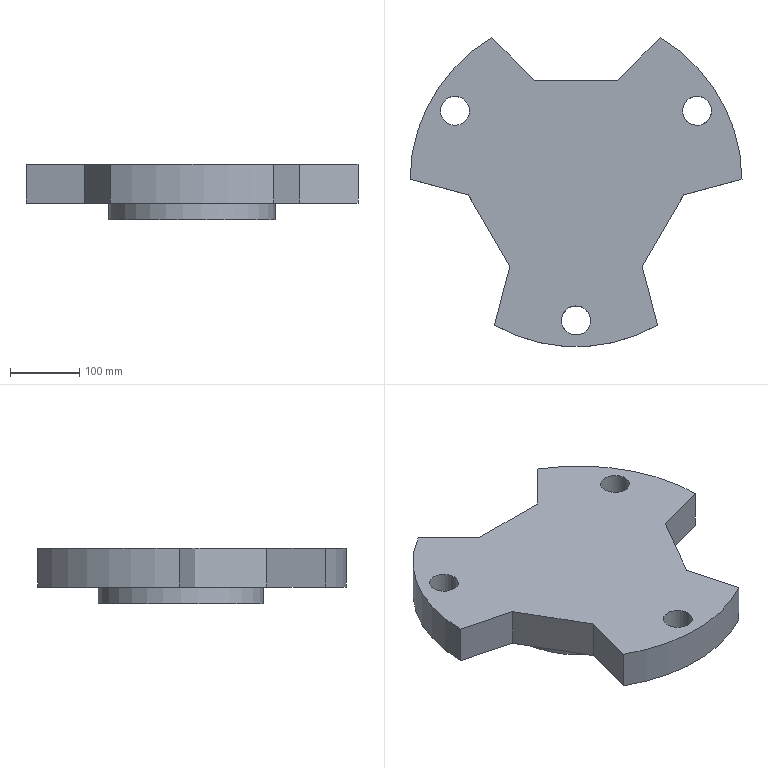Part | NX | features CYLINDER 3, DATUM_CSYS 2, EXTRUDE 1, SKETCH 1 | 1 solid | 21 faces | box 479.982 x 446.798 x 80 mm | volume 8098473 mm3 | plane 13 | cylinder 8 | commonest cylinder face diameters 42 x3 480 x3 48 x1 240 x1
STEP:
#1=CARTESIAN_POINT('',(-239.991,2.081,56.));
#2=VERTEX_POINT('',#1);
#3=CARTESIAN_POINT('',(-239.991,2.081,0.));
#4=VERTEX_POINT('',#3);
#5=CARTESIAN_POINT('',(-239.991,2.081,0.));
#6=DIRECTION('',(0.,0.,1.));
#7=VECTOR('',#6,1000.);
#8=LINE('',#5,#7);
#9=EDGE_CURVE('',#2,#4,#8,.F.);
#10=ORIENTED_EDGE('',*,*,#9,.F.);
#11=CARTESIAN_POINT('',(-121.798,206.798,56.));
#12=VERTEX_POINT('',#11);
#13=CARTESIAN_POINT('',(0.,0.,56.));
#14=DIRECTION('',(0.,0.,-1.));
#15=DIRECTION('',(1.,0.,0.));
#16=AXIS2_PLACEMENT_3D('',#13,#14,#15);
#17=CIRCLE('',#16,240.);
#18=EDGE_CURVE('',#2,#12,#17,.T.);
#19=ORIENTED_EDGE('',*,*,#18,.T.);
#20=CARTESIAN_POINT('',(-121.798,206.798,0.));
#21=VERTEX_POINT('',#20);
#22=CARTESIAN_POINT('',(-121.798,206.798,0.));
#23=DIRECTION('',(0.,0.,1.));
#24=VECTOR('',#23,1000.);
#25=LINE('',#22,#24);
#26=EDGE_CURVE('',#21,#12,#25,.T.);
#27=ORIENTED_EDGE('',*,*,#26,.F.);
#28=CARTESIAN_POINT('',(0.,0.,0.));
#29=DIRECTION('',(0.,0.,1.));
#30=DIRECTION('',(1.,0.,0.));
#31=AXIS2_PLACEMENT_3D('',#28,#29,#30);
#32=CIRCLE('',#31,240.);
#33=EDGE_CURVE('',#21,#4,#32,.T.);
#34=ORIENTED_EDGE('',*,*,#33,.T.);
#35=EDGE_LOOP('',(#10,#19,#27,#34));
#36=FACE_BOUND('',#35,.T.);
#37=CARTESIAN_POINT('',(0.,0.,0.));
#38=DIRECTION('',(0.,0.,1.));
#39=DIRECTION('',(1.,0.,0.));
#40=AXIS2_PLACEMENT_3D('',#37,#38,#39);
#41=CYLINDRICAL_SURFACE('',#40,240.);
#42=ADVANCED_FACE('',(#36),#41,.T.);
#43=CARTESIAN_POINT('',(-118.193,-208.879,0.));
#44=VERTEX_POINT('',#43);
#45=CARTESIAN_POINT('',(-118.193,-208.879,56.));
#46=VERTEX_POINT('',#45);
#47=CARTESIAN_POINT('',(-118.193,-208.879,0.));
#48=DIRECTION('',(0.,0.,1.));
#49=VECTOR('',#48,1000.);
#50=LINE('',#47,#49);
#51=EDGE_CURVE('',#44,#46,#50,.T.);
#52=ORIENTED_EDGE('',*,*,#51,.F.);
#53=CARTESIAN_POINT('',(118.193,-208.879,0.));
#54=VERTEX_POINT('',#53);
#55=CARTESIAN_POINT('',(0.,0.,0.));
#56=DIRECTION('',(0.,0.,1.));
#57=DIRECTION('',(1.,0.,0.));
#58=AXIS2_PLACEMENT_3D('',#55,#56,#57);
#59=CIRCLE('',#58,240.);
#60=EDGE_CURVE('',#44,#54,#59,.T.);
#61=ORIENTED_EDGE('',*,*,#60,.T.);
#62=CARTESIAN_POINT('',(118.193,-208.879,56.));
#63=VERTEX_POINT('',#62);
#64=CARTESIAN_POINT('',(118.193,-208.879,0.));
#65=DIRECTION('',(0.,0.,1.));
#66=VECTOR('',#65,1000.);
#67=LINE('',#64,#66);
#68=EDGE_CURVE('',#63,#54,#67,.F.);
#69=ORIENTED_EDGE('',*,*,#68,.F.);
#70=CARTESIAN_POINT('',(0.,0.,56.));
#71=DIRECTION('',(0.,0.,-1.));
#72=DIRECTION('',(1.,0.,0.));
#73=AXIS2_PLACEMENT_3D('',#70,#71,#72);
#74=CIRCLE('',#73,240.);
#75=EDGE_CURVE('',#63,#46,#74,.T.);
#76=ORIENTED_EDGE('',*,*,#75,.T.);
#77=EDGE_LOOP('',(#52,#61,#69,#76));
#78=FACE_BOUND('',#77,.T.);
#79=CARTESIAN_POINT('',(0.,0.,0.));
#80=DIRECTION('',(0.,0.,1.));
#81=DIRECTION('',(1.,0.,0.));
#82=AXIS2_PLACEMENT_3D('',#79,#80,#81);
#83=CYLINDRICAL_SURFACE('',#82,240.);
#84=ADVANCED_FACE('',(#78),#83,.T.);
#85=CARTESIAN_POINT('',(-154.,101.036,56.));
#86=VERTEX_POINT('',#85);
#87=CARTESIAN_POINT('',(-175.,101.036,56.));
#88=DIRECTION('',(0.,0.,1.));
#89=DIRECTION('',(1.,0.,0.));
#90=AXIS2_PLACEMENT_3D('',#87,#88,#89);
#91=CIRCLE('',#90,21.);
#92=EDGE_CURVE('',#86,#86,#91,.T.);
#93=ORIENTED_EDGE('',*,*,#92,.F.);
#94=EDGE_LOOP('',(#93));
#95=FACE_BOUND('',#94,.T.);
#96=CARTESIAN_POINT('',(-10.5,-183.886,56.));
#97=VERTEX_POINT('',#96);
#98=CARTESIAN_POINT('',(0.,-202.073,56.));
#99=DIRECTION('',(0.,0.,1.));
#100=DIRECTION('',(-0.5,0.866,0.));
#101=AXIS2_PLACEMENT_3D('',#98,#99,#100);
#102=CIRCLE('',#101,21.);
#103=EDGE_CURVE('',#97,#97,#102,.T.);
#104=ORIENTED_EDGE('',*,*,#103,.F.);
#105=EDGE_LOOP('',(#104));
#106=FACE_BOUND('',#105,.T.);
#107=CARTESIAN_POINT('',(164.5,82.85,56.));
#108=VERTEX_POINT('',#107);
#109=CARTESIAN_POINT('',(175.,101.036,56.));
#110=DIRECTION('',(0.,0.,1.));
#111=DIRECTION('',(-0.5,-0.866,0.));
#112=AXIS2_PLACEMENT_3D('',#109,#110,#111);
#113=CIRCLE('',#112,21.);
#114=EDGE_CURVE('',#108,#108,#113,.T.);
#115=ORIENTED_EDGE('',*,*,#114,.F.);
#116=EDGE_LOOP('',(#115));
#117=FACE_BOUND('',#116,.T.);
#118=CARTESIAN_POINT('',(-155.574,-20.538,56.));
#119=VERTEX_POINT('',#118);
#120=CARTESIAN_POINT('',(-155.574,-20.538,56.));
#121=DIRECTION('',(-0.9659,0.2588,0.));
#122=VECTOR('',#121,1000.);
#123=LINE('',#120,#122);
#124=EDGE_CURVE('',#119,#2,#123,.T.);
#125=ORIENTED_EDGE('',*,*,#124,.F.);
#126=CARTESIAN_POINT('',(-95.574,-124.462,56.));
#127=VERTEX_POINT('',#126);
#128=CARTESIAN_POINT('',(-95.574,-124.462,56.));
#129=DIRECTION('',(-0.5,0.866,0.));
#130=VECTOR('',#129,1000.);
#131=LINE('',#128,#130);
#132=EDGE_CURVE('',#127,#119,#131,.T.);
#133=ORIENTED_EDGE('',*,*,#132,.F.);
#134=CARTESIAN_POINT('',(-131.124,-257.136,56.));
#135=DIRECTION('',(0.2588,0.9659,0.));
#136=VECTOR('',#135,1000.);
#137=LINE('',#134,#136);
#138=EDGE_CURVE('',#46,#127,#137,.T.);
#139=ORIENTED_EDGE('',*,*,#138,.F.);
#140=ORIENTED_EDGE('',*,*,#75,.F.);
#141=CARTESIAN_POINT('',(95.574,-124.462,56.));
#142=VERTEX_POINT('',#141);
#143=CARTESIAN_POINT('',(95.574,-124.462,56.));
#144=DIRECTION('',(0.2588,-0.9659,0.));
#145=VECTOR('',#144,1000.);
#146=LINE('',#143,#145);
#147=EDGE_CURVE('',#142,#63,#146,.T.);
#148=ORIENTED_EDGE('',*,*,#147,.F.);
#149=CARTESIAN_POINT('',(155.574,-20.538,56.));
#150=VERTEX_POINT('',#149);
#151=CARTESIAN_POINT('',(155.574,-20.538,56.));
#152=DIRECTION('',(-0.5,-0.866,0.));
#153=VECTOR('',#152,1000.);
#154=LINE('',#151,#153);
#155=EDGE_CURVE('',#150,#142,#154,.T.);
#156=ORIENTED_EDGE('',*,*,#155,.F.);
#157=CARTESIAN_POINT('',(239.991,2.081,56.));
#158=VERTEX_POINT('',#157);
#159=CARTESIAN_POINT('',(288.248,15.011,56.));
#160=DIRECTION('',(-0.9659,-0.2588,0.));
#161=VECTOR('',#160,1000.);
#162=LINE('',#159,#161);
#163=EDGE_CURVE('',#158,#150,#162,.T.);
#164=ORIENTED_EDGE('',*,*,#163,.F.);
#165=CARTESIAN_POINT('',(121.798,206.798,56.));
#166=VERTEX_POINT('',#165);
#167=CARTESIAN_POINT('',(0.,0.,56.));
#168=DIRECTION('',(0.,0.,-1.));
#169=DIRECTION('',(1.,0.,0.));
#170=AXIS2_PLACEMENT_3D('',#167,#168,#169);
#171=CIRCLE('',#170,240.);
#172=EDGE_CURVE('',#166,#158,#171,.T.);
#173=ORIENTED_EDGE('',*,*,#172,.F.);
#174=CARTESIAN_POINT('',(60.,145.,56.));
#175=VERTEX_POINT('',#174);
#176=CARTESIAN_POINT('',(60.,145.,56.));
#177=DIRECTION('',(0.7071,0.7071,0.));
#178=VECTOR('',#177,1000.);
#179=LINE('',#176,#178);
#180=EDGE_CURVE('',#175,#166,#179,.T.);
#181=ORIENTED_EDGE('',*,*,#180,.F.);
#182=CARTESIAN_POINT('',(-60.,145.,56.));
#183=VERTEX_POINT('',#182);
#184=CARTESIAN_POINT('',(-60.,145.,56.));
#185=DIRECTION('',(1.,0.,0.));
#186=VECTOR('',#185,1000.);
#187=LINE('',#184,#186);
#188=EDGE_CURVE('',#183,#175,#187,.T.);
#189=ORIENTED_EDGE('',*,*,#188,.F.);
#190=CARTESIAN_POINT('',(-157.124,242.124,56.));
#191=DIRECTION('',(0.7071,-0.7071,0.));
#192=VECTOR('',#191,1000.);
#193=LINE('',#190,#192);
#194=EDGE_CURVE('',#12,#183,#193,.T.);
#195=ORIENTED_EDGE('',*,*,#194,.F.);
#196=ORIENTED_EDGE('',*,*,#18,.F.);
#197=EDGE_LOOP('',(#125,#133,#139,#140,#148,#156,#164,#173,#181,#189,#195,#196));
#198=FACE_BOUND('',#197,.T.);
#199=CARTESIAN_POINT('',(0.,0.,56.));
#200=DIRECTION('',(0.,0.,1.));
#201=DIRECTION('',(1.,0.,0.));
#202=AXIS2_PLACEMENT_3D('',#199,#200,#201);
#203=PLANE('',#202);
#204=ADVANCED_FACE('',(#95,#106,#117,#198),#203,.T.);
#205=CARTESIAN_POINT('',(-120.,0.,0.));
#206=VERTEX_POINT('',#205);
#207=CARTESIAN_POINT('',(0.,0.,0.));
#208=DIRECTION('',(0.,0.,-1.));
#209=DIRECTION('',(-1.,0.,0.));
#210=AXIS2_PLACEMENT_3D('',#207,#208,#209);
#211=CIRCLE('',#210,120.);
#212=EDGE_CURVE('',#206,#206,#211,.T.);
#213=ORIENTED_EDGE('',*,*,#212,.F.);
#214=EDGE_LOOP('',(#213));
#215=FACE_BOUND('',#214,.T.);
#216=CARTESIAN_POINT('',(-196.,101.036,0.));
#217=VERTEX_POINT('',#216);
#218=CARTESIAN_POINT('',(-175.,101.036,0.));
#219=DIRECTION('',(0.,0.,-1.));
#220=DIRECTION('',(-1.,0.,0.));
#221=AXIS2_PLACEMENT_3D('',#218,#219,#220);
#222=CIRCLE('',#221,21.);
#223=EDGE_CURVE('',#217,#217,#222,.T.);
#224=ORIENTED_EDGE('',*,*,#223,.F.);
#225=EDGE_LOOP('',(#224));
#226=FACE_BOUND('',#225,.T.);
#227=CARTESIAN_POINT('',(-21.,-202.073,0.));
#228=VERTEX_POINT('',#227);
#229=CARTESIAN_POINT('',(0.,-202.073,0.));
#230=DIRECTION('',(0.,0.,-1.));
#231=DIRECTION('',(-1.,0.,0.));
#232=AXIS2_PLACEMENT_3D('',#229,#230,#231);
#233=CIRCLE('',#232,21.);
#234=EDGE_CURVE('',#228,#228,#233,.T.);
#235=ORIENTED_EDGE('',*,*,#234,.F.);
#236=EDGE_LOOP('',(#235));
#237=FACE_BOUND('',#236,.T.);
#238=CARTESIAN_POINT('',(154.,101.036,0.));
#239=VERTEX_POINT('',#238);
#240=CARTESIAN_POINT('',(175.,101.036,0.));
#241=DIRECTION('',(0.,0.,-1.));
#242=DIRECTION('',(-1.,0.,0.));
#243=AXIS2_PLACEMENT_3D('',#240,#241,#242);
#244=CIRCLE('',#243,21.);
#245=EDGE_CURVE('',#239,#239,#244,.T.);
#246=ORIENTED_EDGE('',*,*,#245,.F.);
#247=EDGE_LOOP('',(#246));
#248=FACE_BOUND('',#247,.T.);
#249=CARTESIAN_POINT('',(-155.574,-20.538,0.));
#250=VERTEX_POINT('',#249);
#251=CARTESIAN_POINT('',(-15.556,-58.056,0.));
#252=DIRECTION('',(0.9659,-0.2588,0.));
#253=VECTOR('',#252,1000.);
#254=LINE('',#251,#253);
#255=EDGE_CURVE('',#4,#250,#254,.T.);
#256=ORIENTED_EDGE('',*,*,#255,.F.);
#257=ORIENTED_EDGE('',*,*,#33,.F.);
#258=CARTESIAN_POINT('',(-60.,145.,0.));
#259=VERTEX_POINT('',#258);
#260=CARTESIAN_POINT('',(42.5,42.5,0.));
#261=DIRECTION('',(-0.7071,0.7071,0.));
#262=VECTOR('',#261,1000.);
#263=LINE('',#260,#262);
#264=EDGE_CURVE('',#259,#21,#263,.T.);
#265=ORIENTED_EDGE('',*,*,#264,.F.);
#266=CARTESIAN_POINT('',(60.,145.,0.));
#267=VERTEX_POINT('',#266);
#268=CARTESIAN_POINT('',(0.,145.,0.));
#269=DIRECTION('',(-1.,0.,0.));
#270=VECTOR('',#269,1000.);
#271=LINE('',#268,#270);
#272=EDGE_CURVE('',#267,#259,#271,.T.);
#273=ORIENTED_EDGE('',*,*,#272,.F.);
#274=CARTESIAN_POINT('',(121.798,206.798,0.));
#275=VERTEX_POINT('',#274);
#276=CARTESIAN_POINT('',(-42.5,42.5,0.));
#277=DIRECTION('',(-0.7071,-0.7071,0.));
#278=VECTOR('',#277,1000.);
#279=LINE('',#276,#278);
#280=EDGE_CURVE('',#275,#267,#279,.T.);
#281=ORIENTED_EDGE('',*,*,#280,.F.);
#282=CARTESIAN_POINT('',(239.991,2.081,0.));
#283=VERTEX_POINT('',#282);
#284=CARTESIAN_POINT('',(0.,0.,0.));
#285=DIRECTION('',(0.,0.,1.));
#286=DIRECTION('',(1.,0.,0.));
#287=AXIS2_PLACEMENT_3D('',#284,#285,#286);
#288=CIRCLE('',#287,240.);
#289=EDGE_CURVE('',#283,#275,#288,.T.);
#290=ORIENTED_EDGE('',*,*,#289,.F.);
#291=CARTESIAN_POINT('',(155.574,-20.538,0.));
#292=VERTEX_POINT('',#291);
#293=CARTESIAN_POINT('',(15.556,-58.056,0.));
#294=DIRECTION('',(0.9659,0.2588,0.));
#295=VECTOR('',#294,1000.);
#296=LINE('',#293,#295);
#297=EDGE_CURVE('',#292,#283,#296,.T.);
#298=ORIENTED_EDGE('',*,*,#297,.F.);
#299=CARTESIAN_POINT('',(95.574,-124.462,0.));
#300=VERTEX_POINT('',#299);
#301=CARTESIAN_POINT('',(125.574,-72.5,0.));
#302=DIRECTION('',(0.5,0.866,0.));
#303=VECTOR('',#302,1000.);
#304=LINE('',#301,#303);
#305=EDGE_CURVE('',#300,#292,#304,.T.);
#306=ORIENTED_EDGE('',*,*,#305,.F.);
#307=CARTESIAN_POINT('',(58.056,15.556,0.));
#308=DIRECTION('',(-0.2588,0.9659,0.));
#309=VECTOR('',#308,1000.);
#310=LINE('',#307,#309);
#311=EDGE_CURVE('',#54,#300,#310,.T.);
#312=ORIENTED_EDGE('',*,*,#311,.F.);
#313=ORIENTED_EDGE('',*,*,#60,.F.);
#314=CARTESIAN_POINT('',(-95.574,-124.462,0.));
#315=VERTEX_POINT('',#314);
#316=CARTESIAN_POINT('',(-58.056,15.556,0.));
#317=DIRECTION('',(-0.2588,-0.9659,0.));
#318=VECTOR('',#317,1000.);
#319=LINE('',#316,#318);
#320=EDGE_CURVE('',#315,#44,#319,.T.);
#321=ORIENTED_EDGE('',*,*,#320,.F.);
#322=CARTESIAN_POINT('',(-125.574,-72.5,0.));
#323=DIRECTION('',(0.5,-0.866,0.));
#324=VECTOR('',#323,1000.);
#325=LINE('',#322,#324);
#326=EDGE_CURVE('',#250,#315,#325,.T.);
#327=ORIENTED_EDGE('',*,*,#326,.F.);
#328=EDGE_LOOP('',(#256,#257,#265,#273,#281,#290,#298,#306,#312,#313,#321,#327));
#329=FACE_BOUND('',#328,.T.);
#330=CARTESIAN_POINT('',(0.,0.,0.));
#331=DIRECTION('',(0.,0.,-1.));
#332=DIRECTION('',(-1.,0.,0.));
#333=AXIS2_PLACEMENT_3D('',#330,#331,#332);
#334=PLANE('',#333);
#335=ADVANCED_FACE('',(#215,#226,#237,#248,#329),#334,.T.);
#336=CARTESIAN_POINT('',(121.798,206.798,0.));
#337=DIRECTION('',(0.,0.,1.));
#338=VECTOR('',#337,1000.);
#339=LINE('',#336,#338);
#340=EDGE_CURVE('',#166,#275,#339,.F.);
#341=ORIENTED_EDGE('',*,*,#340,.F.);
#342=ORIENTED_EDGE('',*,*,#172,.T.);
#343=CARTESIAN_POINT('',(239.991,2.081,0.));
#344=DIRECTION('',(0.,0.,1.));
#345=VECTOR('',#344,1000.);
#346=LINE('',#343,#345);
#347=EDGE_CURVE('',#283,#158,#346,.T.);
#348=ORIENTED_EDGE('',*,*,#347,.F.);
#349=ORIENTED_EDGE('',*,*,#289,.T.);
#350=EDGE_LOOP('',(#341,#342,#348,#349));
#351=FACE_BOUND('',#350,.T.);
#352=CARTESIAN_POINT('',(0.,0.,0.));
#353=DIRECTION('',(0.,0.,1.));
#354=DIRECTION('',(1.,0.,0.));
#355=AXIS2_PLACEMENT_3D('',#352,#353,#354);
#356=CYLINDRICAL_SURFACE('',#355,240.);
#357=ADVANCED_FACE('',(#351),#356,.T.);
#358=ORIENTED_EDGE('',*,*,#311,.T.);
#359=CARTESIAN_POINT('',(95.574,-124.462,-19.));
#360=DIRECTION('',(0.,0.,1.));
#361=VECTOR('',#360,1000.);
#362=LINE('',#359,#361);
#363=EDGE_CURVE('',#142,#300,#362,.F.);
#364=ORIENTED_EDGE('',*,*,#363,.F.);
#365=ORIENTED_EDGE('',*,*,#147,.T.);
#366=ORIENTED_EDGE('',*,*,#68,.T.);
#367=EDGE_LOOP('',(#358,#364,#365,#366));
#368=FACE_BOUND('',#367,.T.);
#369=CARTESIAN_POINT('',(95.574,-124.462,-19.));
#370=DIRECTION('',(-0.9659,-0.2588,0.));
#371=DIRECTION('',(0.2588,-0.9659,0.));
#372=AXIS2_PLACEMENT_3D('',#369,#370,#371);
#373=PLANE('',#372);
#374=ADVANCED_FACE('',(#368),#373,.F.);
#375=ORIENTED_EDGE('',*,*,#297,.T.);
#376=ORIENTED_EDGE('',*,*,#347,.T.);
#377=ORIENTED_EDGE('',*,*,#163,.T.);
#378=CARTESIAN_POINT('',(155.574,-20.538,-19.));
#379=DIRECTION('',(0.,0.,1.));
#380=VECTOR('',#379,1000.);
#381=LINE('',#378,#380);
#382=EDGE_CURVE('',#150,#292,#381,.F.);
#383=ORIENTED_EDGE('',*,*,#382,.T.);
#384=EDGE_LOOP('',(#375,#376,#377,#383));
#385=FACE_BOUND('',#384,.T.);
#386=CARTESIAN_POINT('',(288.248,15.011,-19.));
#387=DIRECTION('',(-0.2588,0.9659,0.));
#388=DIRECTION('',(-0.9659,-0.2588,0.));
#389=AXIS2_PLACEMENT_3D('',#386,#387,#388);
#390=PLANE('',#389);
#391=ADVANCED_FACE('',(#385),#390,.F.);
#392=ORIENTED_EDGE('',*,*,#305,.T.);
#393=ORIENTED_EDGE('',*,*,#382,.F.);
#394=ORIENTED_EDGE('',*,*,#155,.T.);
#395=ORIENTED_EDGE('',*,*,#363,.T.);
#396=EDGE_LOOP('',(#392,#393,#394,#395));
#397=FACE_BOUND('',#396,.T.);
#398=CARTESIAN_POINT('',(155.574,-20.538,-19.));
#399=DIRECTION('',(-0.866,0.5,0.));
#400=DIRECTION('',(-0.5,-0.866,0.));
#401=AXIS2_PLACEMENT_3D('',#398,#399,#400);
#402=PLANE('',#401);
#403=ADVANCED_FACE('',(#397),#402,.F.);
#404=ORIENTED_EDGE('',*,*,#264,.T.);
#405=ORIENTED_EDGE('',*,*,#26,.T.);
#406=ORIENTED_EDGE('',*,*,#194,.T.);
#407=CARTESIAN_POINT('',(-60.,145.,-19.));
#408=DIRECTION('',(0.,0.,1.));
#409=VECTOR('',#408,1000.);
#410=LINE('',#407,#409);
#411=EDGE_CURVE('',#183,#259,#410,.F.);
#412=ORIENTED_EDGE('',*,*,#411,.T.);
#413=EDGE_LOOP('',(#404,#405,#406,#412));
#414=FACE_BOUND('',#413,.T.);
#415=CARTESIAN_POINT('',(-157.124,242.124,-19.));
#416=DIRECTION('',(-0.7071,-0.7071,0.));
#417=DIRECTION('',(0.7071,-0.7071,0.));
#418=AXIS2_PLACEMENT_3D('',#415,#416,#417);
#419=PLANE('',#418);
#420=ADVANCED_FACE('',(#414),#419,.F.);
#421=ORIENTED_EDGE('',*,*,#272,.T.);
#422=ORIENTED_EDGE('',*,*,#411,.F.);
#423=ORIENTED_EDGE('',*,*,#188,.T.);
#424=CARTESIAN_POINT('',(60.,145.,-19.));
#425=DIRECTION('',(0.,0.,1.));
#426=VECTOR('',#425,1000.);
#427=LINE('',#424,#426);
#428=EDGE_CURVE('',#175,#267,#427,.F.);
#429=ORIENTED_EDGE('',*,*,#428,.T.);
#430=EDGE_LOOP('',(#421,#422,#423,#429));
#431=FACE_BOUND('',#430,.T.);
#432=CARTESIAN_POINT('',(-60.,145.,-19.));
#433=DIRECTION('',(0.,-1.,0.));
#434=DIRECTION('',(0.,0.,-1.));
#435=AXIS2_PLACEMENT_3D('',#432,#433,#434);
#436=PLANE('',#435);
#437=ADVANCED_FACE('',(#431),#436,.F.);
#438=ORIENTED_EDGE('',*,*,#280,.T.);
#439=ORIENTED_EDGE('',*,*,#428,.F.);
#440=ORIENTED_EDGE('',*,*,#180,.T.);
#441=ORIENTED_EDGE('',*,*,#340,.T.);
#442=EDGE_LOOP('',(#438,#439,#440,#441));
#443=FACE_BOUND('',#442,.T.);
#444=CARTESIAN_POINT('',(60.,145.,-19.));
#445=DIRECTION('',(0.7071,-0.7071,0.));
#446=DIRECTION('',(0.7071,0.7071,0.));
#447=AXIS2_PLACEMENT_3D('',#444,#445,#446);
#448=PLANE('',#447);
#449=ADVANCED_FACE('',(#443),#448,.F.);
#450=ORIENTED_EDGE('',*,*,#9,.T.);
#451=ORIENTED_EDGE('',*,*,#255,.T.);
#452=CARTESIAN_POINT('',(-155.574,-20.538,-19.));
#453=DIRECTION('',(0.,0.,1.));
#454=VECTOR('',#453,1000.);
#455=LINE('',#452,#454);
#456=EDGE_CURVE('',#119,#250,#455,.F.);
#457=ORIENTED_EDGE('',*,*,#456,.F.);
#458=ORIENTED_EDGE('',*,*,#124,.T.);
#459=EDGE_LOOP('',(#450,#451,#457,#458));
#460=FACE_BOUND('',#459,.T.);
#461=CARTESIAN_POINT('',(-155.574,-20.538,-19.));
#462=DIRECTION('',(0.2588,0.9659,0.));
#463=DIRECTION('',(-0.9659,0.2588,0.));
#464=AXIS2_PLACEMENT_3D('',#461,#462,#463);
#465=PLANE('',#464);
#466=ADVANCED_FACE('',(#460),#465,.F.);
#467=ORIENTED_EDGE('',*,*,#51,.T.);
#468=ORIENTED_EDGE('',*,*,#138,.T.);
#469=CARTESIAN_POINT('',(-95.574,-124.462,-19.));
#470=DIRECTION('',(0.,0.,1.));
#471=VECTOR('',#470,1000.);
#472=LINE('',#469,#471);
#473=EDGE_CURVE('',#127,#315,#472,.F.);
#474=ORIENTED_EDGE('',*,*,#473,.T.);
#475=ORIENTED_EDGE('',*,*,#320,.T.);
#476=EDGE_LOOP('',(#467,#468,#474,#475));
#477=FACE_BOUND('',#476,.T.);
#478=CARTESIAN_POINT('',(-131.124,-257.136,-19.));
#479=DIRECTION('',(0.9659,-0.2588,0.));
#480=DIRECTION('',(0.2588,0.9659,0.));
#481=AXIS2_PLACEMENT_3D('',#478,#479,#480);
#482=PLANE('',#481);
#483=ADVANCED_FACE('',(#477),#482,.F.);
#484=ORIENTED_EDGE('',*,*,#326,.T.);
#485=ORIENTED_EDGE('',*,*,#473,.F.);
#486=ORIENTED_EDGE('',*,*,#132,.T.);
#487=ORIENTED_EDGE('',*,*,#456,.T.);
#488=EDGE_LOOP('',(#484,#485,#486,#487));
#489=FACE_BOUND('',#488,.T.);
#490=CARTESIAN_POINT('',(-95.574,-124.462,-19.));
#491=DIRECTION('',(0.866,0.5,0.));
#492=DIRECTION('',(-0.5,0.866,0.));
#493=AXIS2_PLACEMENT_3D('',#490,#491,#492);
#494=PLANE('',#493);
#495=ADVANCED_FACE('',(#489),#494,.F.);
#496=ORIENTED_EDGE('',*,*,#245,.T.);
#497=EDGE_LOOP('',(#496));
#498=FACE_BOUND('',#497,.T.);
#499=ORIENTED_EDGE('',*,*,#114,.T.);
#500=EDGE_LOOP('',(#499));
#501=FACE_BOUND('',#500,.T.);
#502=CARTESIAN_POINT('',(175.,101.036,-19.));
#503=DIRECTION('',(0.,0.,1.));
#504=DIRECTION('',(1.,0.,0.));
#505=AXIS2_PLACEMENT_3D('',#502,#503,#504);
#506=CYLINDRICAL_SURFACE('',#505,21.);
#507=ADVANCED_FACE('',(#498,#501),#506,.F.);
#508=ORIENTED_EDGE('',*,*,#234,.T.);
#509=EDGE_LOOP('',(#508));
#510=FACE_BOUND('',#509,.T.);
#511=ORIENTED_EDGE('',*,*,#103,.T.);
#512=EDGE_LOOP('',(#511));
#513=FACE_BOUND('',#512,.T.);
#514=CARTESIAN_POINT('',(0.,-202.073,-19.));
#515=DIRECTION('',(0.,0.,1.));
#516=DIRECTION('',(1.,0.,0.));
#517=AXIS2_PLACEMENT_3D('',#514,#515,#516);
#518=CYLINDRICAL_SURFACE('',#517,21.);
#519=ADVANCED_FACE('',(#510,#513),#518,.F.);
#520=ORIENTED_EDGE('',*,*,#223,.T.);
#521=EDGE_LOOP('',(#520));
#522=FACE_BOUND('',#521,.T.);
#523=ORIENTED_EDGE('',*,*,#92,.T.);
#524=EDGE_LOOP('',(#523));
#525=FACE_BOUND('',#524,.T.);
#526=CARTESIAN_POINT('',(-175.,101.036,-19.));
#527=DIRECTION('',(0.,0.,1.));
#528=DIRECTION('',(1.,0.,0.));
#529=AXIS2_PLACEMENT_3D('',#526,#527,#528);
#530=CYLINDRICAL_SURFACE('',#529,21.);
#531=ADVANCED_FACE('',(#522,#525),#530,.F.);
#532=CARTESIAN_POINT('',(24.,0.,-24.));
#533=VERTEX_POINT('',#532);
#534=CARTESIAN_POINT('',(0.,0.,-24.));
#535=DIRECTION('',(0.,0.,1.));
#536=DIRECTION('',(1.,0.,0.));
#537=AXIS2_PLACEMENT_3D('',#534,#535,#536);
#538=CIRCLE('',#537,24.);
#539=EDGE_CURVE('',#533,#533,#538,.T.);
#540=ORIENTED_EDGE('',*,*,#539,.T.);
#541=EDGE_LOOP('',(#540));
#542=FACE_BOUND('',#541,.T.);
#543=CARTESIAN_POINT('',(120.,0.,-24.));
#544=VERTEX_POINT('',#543);
#545=CARTESIAN_POINT('',(0.,0.,-24.));
#546=DIRECTION('',(0.,0.,1.));
#547=DIRECTION('',(1.,0.,0.));
#548=AXIS2_PLACEMENT_3D('',#545,#546,#547);
#549=CIRCLE('',#548,120.);
#550=EDGE_CURVE('',#544,#544,#549,.T.);
#551=ORIENTED_EDGE('',*,*,#550,.F.);
#552=EDGE_LOOP('',(#551));
#553=FACE_BOUND('',#552,.T.);
#554=CARTESIAN_POINT('',(0.,0.,-24.));
#555=DIRECTION('',(0.,0.,-1.));
#556=DIRECTION('',(-1.,0.,0.));
#557=AXIS2_PLACEMENT_3D('',#554,#555,#556);
#558=PLANE('',#557);
#559=ADVANCED_FACE('',(#542,#553),#558,.T.);
#560=ORIENTED_EDGE('',*,*,#550,.T.);
#561=EDGE_LOOP('',(#560));
#562=FACE_BOUND('',#561,.T.);
#563=ORIENTED_EDGE('',*,*,#212,.T.);
#564=EDGE_LOOP('',(#563));
#565=FACE_BOUND('',#564,.T.);
#566=CARTESIAN_POINT('',(0.,0.,0.));
#567=DIRECTION('',(0.,0.,-1.));
#568=DIRECTION('',(1.,0.,0.));
#569=AXIS2_PLACEMENT_3D('',#566,#567,#568);
#570=CYLINDRICAL_SURFACE('',#569,120.);
#571=ADVANCED_FACE('',(#562,#565),#570,.T.);
#572=CARTESIAN_POINT('',(24.,0.,21.));
#573=VERTEX_POINT('',#572);
#574=CARTESIAN_POINT('',(0.,0.,21.));
#575=DIRECTION('',(0.,0.,-1.));
#576=DIRECTION('',(1.,0.,0.));
#577=AXIS2_PLACEMENT_3D('',#574,#575,#576);
#578=CIRCLE('',#577,24.);
#579=EDGE_CURVE('',#573,#573,#578,.F.);
#580=ORIENTED_EDGE('',*,*,#579,.F.);
#581=EDGE_LOOP('',(#580));
#582=FACE_BOUND('',#581,.T.);
#583=CARTESIAN_POINT('',(0.,0.,21.));
#584=DIRECTION('',(0.,0.,1.));
#585=DIRECTION('',(1.,0.,0.));
#586=AXIS2_PLACEMENT_3D('',#583,#584,#585);
#587=PLANE('',#586);
#588=ADVANCED_FACE('',(#582),#587,.F.);
#589=ORIENTED_EDGE('',*,*,#579,.T.);
#590=EDGE_LOOP('',(#589));
#591=FACE_BOUND('',#590,.T.);
#592=ORIENTED_EDGE('',*,*,#539,.F.);
#593=EDGE_LOOP('',(#592));
#594=FACE_BOUND('',#593,.T.);
#595=CARTESIAN_POINT('',(0.,0.,-24.));
#596=DIRECTION('',(0.,0.,1.));
#597=DIRECTION('',(1.,0.,0.));
#598=AXIS2_PLACEMENT_3D('',#595,#596,#597);
#599=CYLINDRICAL_SURFACE('',#598,24.);
#600=ADVANCED_FACE('',(#591,#594),#599,.F.);
#601=CLOSED_SHELL('',(#42,#84,#204,#335,#357,#374,#391,#403,#420,#437,#449,#466,#483,#495,#507,#519,#531,#559,#571,#588,#600));
#602=MANIFOLD_SOLID_BREP('',#601);
#603=(LENGTH_UNIT()NAMED_UNIT(*)SI_UNIT(.MILLI.,.METRE.));
#604=UNCERTAINTY_MEASURE_WITH_UNIT(LENGTH_MEASURE(0.00001),#603,'','');
#605=(NAMED_UNIT(*)PLANE_ANGLE_UNIT()SI_UNIT($,.RADIAN.));
#606=(NAMED_UNIT(*)SI_UNIT($,.STERADIAN.)SOLID_ANGLE_UNIT());
#607=(GEOMETRIC_REPRESENTATION_CONTEXT(3)GLOBAL_UNCERTAINTY_ASSIGNED_CONTEXT((#604))GLOBAL_UNIT_ASSIGNED_CONTEXT((#603,#605,#606))REPRESENTATION_CONTEXT('',''));
#608=ADVANCED_BREP_SHAPE_REPRESENTATION('',(#602),#607);